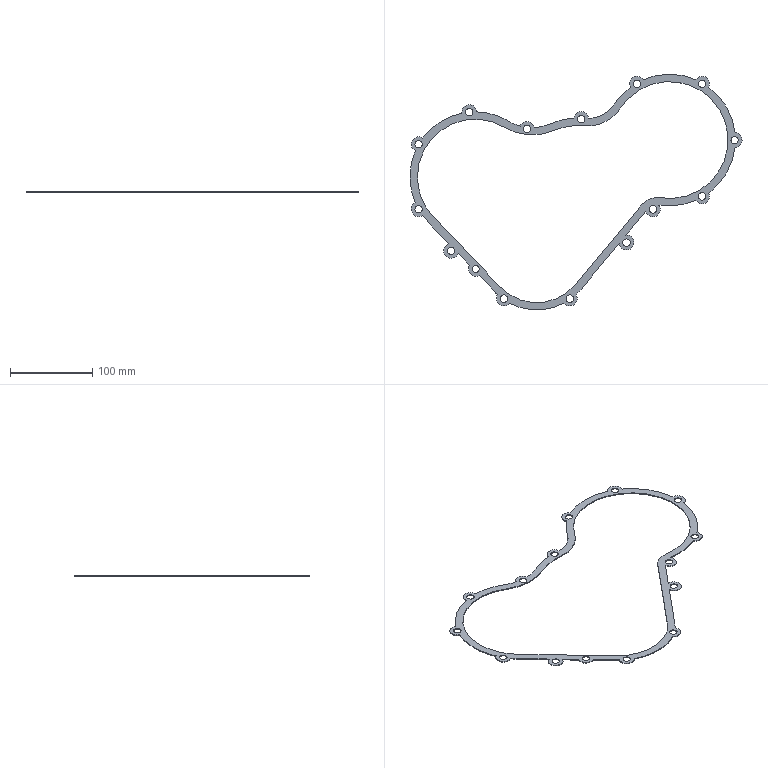Part | SolidWorks | features BaseBody 1 | 1 solid | 86 faces | box 403.3 x 286.5 x 1 mm | volume 10528 mm3 | cylinder 77 | plane 9 | commonest cylinder face diameters 9 x28 18 x22 140 x5 158 x5 160 x5 8.5 x2